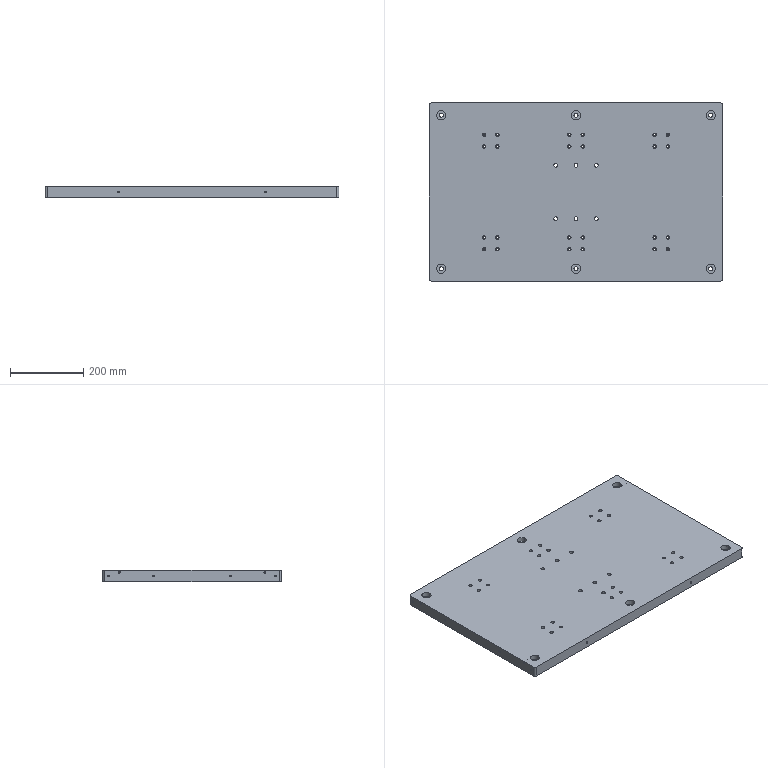NC program | Mastercam | posted with a generic post | part box 800 x 485 x 30 mm
Lines 1 to 630 of 13355:
%
O0000()
(MATERIAL - ALUMINUM MM - 2024)
( T9 | 10 FEM | H9 | XY STOCK TO LEAVE - .2 | Z STOCK TO LEAVE - .05 )
( T10 | 10 FEM | H10 | XY STOCK TO LEAVE - 0. | Z STOCK TO LEAVE - .05 )
( T7 | 6 CHM | H7 )
( T20 | 20 FEM | H20 | XY STOCK TO LEAVE - .15 | Z STOCK TO LEAVE - .1 )
( T1 | 6.8 DR | H1 )
( T18 | 8 DR | H18 )
( T24 | 100 FEM | H24 | XY STOCK TO LEAVE - -1. | Z STOCK TO LEAVE - 0. )
N100 G21
N110 G0 G17 G40 G49 G80 G90
( LRRE )
N120 T9 M6
N130 G0 G90 G54 X-410. Y180.2 A0. S7000 M3
N140 G43 H9 Z50. M8
N150 Z1.
N160 G1 Z-.998 F600.
N170 X-390. F3000.
N180 X-5.
N190 X390.
N200 X410.
N210 Z-1.995 F600.
N220 X390. F3000.
N230 X-5.
N240 X-390.
N250 X-410.
N260 Z-2.993 F600.
N270 X-390. F3000.
N280 X-5.
N290 X390.
N300 X410.
N310 Z-3.99 F600.
N320 X390. F3000.
N330 X-5.
N340 X-390.
N350 X-410.
N360 Z-4.987 F600.
N370 X-390. F3000.
N380 X-5.
N390 X390.
N400 X410.
N410 Z-5.985 F600.
N420 X390. F3000.
N430 X-5.
N440 X-390.
N450 X-410.
N460 Z-6.982 F600.
N470 X-390. F3000.
N480 X-5.
N490 X390.
N500 X410.
N510 Z-7.98 F600.
N520 X390. F3000.
N530 X-5.
N540 X-390.
N550 X-410.
N560 Z-8.977 F600.
N570 X-390. F3000.
N580 X-5.
N590 X390.
N600 X410.
N610 Z-9.975 F600.
N620 X390. F3000.
N630 X-5.
N640 X-390.
N650 X-410.
N660 Z-10.973 F600.
N670 X-390. F3000.
N680 X-5.
N690 X390.
N700 X410.
N710 Z-11.97 F600.
N720 X390. F3000.
N730 X-5.
N740 X-390.
N750 X-410.
N760 Z-12.967 F600.
N770 X-390. F3000.
N780 X-5.
N790 X390.
N800 X410.
N810 Z-13.965 F600.
N820 X390. F3000.
N830 X-5.
N840 X-390.
N850 X-410.
N860 Z-14.963 F600.
N870 X-390. F3000.
N880 X-5.
N890 X390.
N900 X410.
N910 Z-15.96 F600.
N920 X390. F3000.
N930 X-5.
N940 X-390.
N950 X-410.
N960 Z-16.957 F600.
N970 X-390. F3000.
N980 X-5.
N990 X390.
N1000 X410.
N1010 Z-17.955 F600.
N1020 X390. F3000.
N1030 X-5.
N1040 X-390.
N1050 X-410.
N1060 Z-18.953 F600.
N1070 X-390. F3000.
N1080 X-5.
N1090 X390.
N1100 X410.
N1110 Z-19.95 F600.
N1120 X390. F3000.
N1130 X-5.
N1140 X-390.
N1150 X-410.
N1160 G0 Z50.
N1170 X410. Y-180.2
N1180 Z1.
N1190 G1 Z-.998 F600.
N1200 X390. F3000.
N1210 X-5.
N1220 X-390.
N1230 X-410.
N1240 Z-1.995 F600.
N1250 X-390. F3000.
N1260 X-5.
N1270 X390.
N1280 X410.
N1290 Z-2.993 F600.
N1300 X390. F3000.
N1310 X-5.
N1320 X-390.
N1330 X-410.
N1340 Z-3.99 F600.
N1350 X-390. F3000.
N1360 X-5.
N1370 X390.
N1380 X410.
N1390 Z-4.987 F600.
N1400 X390. F3000.
N1410 X-5.
N1420 X-390.
N1430 X-410.
N1440 Z-5.985 F600.
N1450 X-390. F3000.
N1460 X-5.
N1470 X390.
N1480 X410.
N1490 Z-6.982 F600.
N1500 X390. F3000.
N1510 X-5.
N1520 X-390.
N1530 X-410.
N1540 Z-7.98 F600.
N1550 X-390. F3000.
N1560 X-5.
N1570 X390.
N1580 X410.
N1590 Z-8.977 F600.
N1600 X390. F3000.
N1610 X-5.
N1620 X-390.
N1630 X-410.
N1640 Z-9.975 F600.
N1650 X-390. F3000.
N1660 X-5.
N1670 X390.
N1680 X410.
N1690 Z-10.973 F600.
N1700 X390. F3000.
N1710 X-5.
N1720 X-390.
N1730 X-410.
N1740 Z-11.97 F600.
N1750 X-390. F3000.
N1760 X-5.
N1770 X390.
N1780 X410.
N1790 Z-12.967 F600.
N1800 X390. F3000.
N1810 X-5.
N1820 X-390.
N1830 X-410.
N1840 Z-13.965 F600.
N1850 X-390. F3000.
N1860 X-5.
N1870 X390.
N1880 X410.
N1890 Z-14.963 F600.
N1900 X390. F3000.
N1910 X-5.
N1920 X-390.
N1930 X-410.
N1940 Z-15.96 F600.
N1950 X-390. F3000.
N1960 X-5.
N1970 X390.
N1980 X410.
N1990 Z-16.957 F600.
N2000 X390. F3000.
N2010 X-5.
N2020 X-390.
N2030 X-410.
N2040 Z-17.955 F600.
N2050 X-390. F3000.
N2060 X-5.
N2070 X390.
N2080 X410.
N2090 Z-18.953 F600.
N2100 X390. F3000.
N2110 X-5.
N2120 X-390.
N2130 X-410.
N2140 Z-19.95 F600.
N2150 X-390. F3000.
N2160 X-5.
N2170 X390.
N2180 X410.
N2190 G0 Z50.
N2200 M5
N2210 G91 G28 Z0. M9
N2220 A0.
N2230 M01
N2240 T10 M6
N2250 G0 G90 G17 G54 X-410. Y180. A0. S7000 M3
N2260 G43 H10 Z50. M8
N2270 Z1.
N2280 G1 Z-19.95 F600.
N2290 X-390. F1000.
N2300 X-5.
N2310 X390.
N2320 X410.
N2330 G0 Z50.
N2340 Y-180.
N2350 Z1.
N2360 G1 Z-19.95 F600.
N2370 X390. F1000.
N2380 X-5.
N2390 X-390.
N2400 X-410.
N2410 G0 Z50.
N2420 M5
N2430 G91 G28 Z0. M9
N2440 A0.
N2450 M01
N2460 T7 M6
N2470 G0 G90 G17 G54 X-410. Y175.65 A0. S7000 M3
N2480 G43 H7 Z50. M8
N2490 Z1.
N2500 G1 Z-.8 F600.
N2510 X-390. F1000.
N2520 X-5.
N2530 X390.
N2540 X410.
N2550 G0 Z50.
N2560 Y-175.65
N2570 Z1.
N2580 G1 Z-.8 F600.
N2590 X390. F1000.
N2600 X-5.
N2610 X-390.
N2620 X-410.
N2630 G0 Z50.
N2640 M5
N2650 G91 G28 Z0. M9
N2660 A0.
N2670 M01
( LRRECFRBL )
N2680 T9 M6
N2690 G0 G90 G17 G54 X-388. Y-184.2 A0. S7000 M3
N2700 G43 H9 Z50. M8
N2710 Z1.
N2720 G1 Z-.998 F600.
N2730 Y-182.2 F3000.
N2740 G3 X-390. Y-180.2 I-2. J0.
N2750 G2 X-400.2 Y-170. I0. J10.2
N2760 G1 Y170.
N2770 G2 X-390. Y180.2 I10.2 J0.
N2780 G3 X-388. Y182.2 I0. J2.
N2790 G1 Y184.2
N2800 Z-1.995 F600.
N2810 Y182.2 F3000.
N2820 G2 X-390. Y180.2 I-2. J0.
N2830 G3 X-400.2 Y170. I0. J-10.2
N2840 G1 Y-170.
N2850 G3 X-390. Y-180.2 I10.2 J0.
N2860 G2 X-388. Y-182.2 I0. J-2.
N2870 G1 Y-184.2
N2880 Z-2.993 F600.
N2890 Y-182.2 F3000.
N2900 G3 X-390. Y-180.2 I-2. J0.
N2910 G2 X-400.2 Y-170. I0. J10.2
N2920 G1 Y170.
N2930 G2 X-390. Y180.2 I10.2 J0.
N2940 G3 X-388. Y182.2 I0. J2.
N2950 G1 Y184.2
N2960 Z-3.99 F600.
N2970 Y182.2 F3000.
N2980 G2 X-390. Y180.2 I-2. J0.
N2990 G3 X-400.2 Y170. I0. J-10.2
N3000 G1 Y-170.
N3010 G3 X-390. Y-180.2 I10.2 J0.
N3020 G2 X-388. Y-182.2 I0. J-2.
N3030 G1 Y-184.2
N3040 Z-4.987 F600.
N3050 Y-182.2 F3000.
N3060 G3 X-390. Y-180.2 I-2. J0.
N3070 G2 X-400.2 Y-170. I0. J10.2
N3080 G1 Y170.
N3090 G2 X-390. Y180.2 I10.2 J0.
N3100 G3 X-388. Y182.2 I0. J2.
N3110 G1 Y184.2
N3120 Z-5.985 F600.
N3130 Y182.2 F3000.
N3140 G2 X-390. Y180.2 I-2. J0.
N3150 G3 X-400.2 Y170. I0. J-10.2
N3160 G1 Y-170.
N3170 G3 X-390. Y-180.2 I10.2 J0.
N3180 G2 X-388. Y-182.2 I0. J-2.
N3190 G1 Y-184.2
N3200 Z-6.982 F600.
N3210 Y-182.2 F3000.
N3220 G3 X-390. Y-180.2 I-2. J0.
N3230 G2 X-400.2 Y-170. I0. J10.2
N3240 G1 Y170.
N3250 G2 X-390. Y180.2 I10.2 J0.
N3260 G3 X-388. Y182.2 I0. J2.
N3270 G1 Y184.2
N3280 Z-7.98 F600.
N3290 Y182.2 F3000.
N3300 G2 X-390. Y180.2 I-2. J0.
N3310 G3 X-400.2 Y170. I0. J-10.2
N3320 G1 Y-170.
N3330 G3 X-390. Y-180.2 I10.2 J0.
N3340 G2 X-388. Y-182.2 I0. J-2.
N3350 G1 Y-184.2
N3360 Z-8.977 F600.
N3370 Y-182.2 F3000.
N3380 G3 X-390. Y-180.2 I-2. J0.
N3390 G2 X-400.2 Y-170. I0. J10.2
N3400 G1 Y170.
N3410 G2 X-390. Y180.2 I10.2 J0.
N3420 G3 X-388. Y182.2 I0. J2.
N3430 G1 Y184.2
N3440 Z-9.975 F600.
N3450 Y182.2 F3000.
N3460 G2 X-390. Y180.2 I-2. J0.
N3470 G3 X-400.2 Y170. I0. J-10.2
N3480 G1 Y-170.
N3490 G3 X-390. Y-180.2 I10.2 J0.
N3500 G2 X-388. Y-182.2 I0. J-2.
N3510 G1 Y-184.2
N3520 Z-10.973 F600.
N3530 Y-182.2 F3000.
N3540 G3 X-390. Y-180.2 I-2. J0.
N3550 G2 X-400.2 Y-170. I0. J10.2
N3560 G1 Y170.
N3570 G2 X-390. Y180.2 I10.2 J0.
N3580 G3 X-388. Y182.2 I0. J2.
N3590 G1 Y184.2
N3600 Z-11.97 F600.
N3610 Y182.2 F3000.
N3620 G2 X-390. Y180.2 I-2. J0.
N3630 G3 X-400.2 Y170. I0. J-10.2
N3640 G1 Y-170.
N3650 G3 X-390. Y-180.2 I10.2 J0.
N3660 G2 X-388. Y-182.2 I0. J-2.
N3670 G1 Y-184.2
N3680 Z-12.967 F600.
N3690 Y-182.2 F3000.
N3700 G3 X-390. Y-180.2 I-2. J0.
N3710 G2 X-400.2 Y-170. I0. J10.2
N3720 G1 Y170.
N3730 G2 X-390. Y180.2 I10.2 J0.
N3740 G3 X-388. Y182.2 I0. J2.
N3750 G1 Y184.2
N3760 Z-13.965 F600.
N3770 Y182.2 F3000.
N3780 G2 X-390. Y180.2 I-2. J0.
N3790 G3 X-400.2 Y170. I0. J-10.2
N3800 G1 Y-170.
N3810 G3 X-390. Y-180.2 I10.2 J0.
N3820 G2 X-388. Y-182.2 I0. J-2.
N3830 G1 Y-184.2
N3840 Z-14.963 F600.
N3850 Y-182.2 F3000.
N3860 G3 X-390. Y-180.2 I-2. J0.
N3870 G2 X-400.2 Y-170. I0. J10.2
N3880 G1 Y170.
N3890 G2 X-390. Y180.2 I10.2 J0.
N3900 G3 X-388. Y182.2 I0. J2.
N3910 G1 Y184.2
N3920 Z-15.96 F600.
N3930 Y182.2 F3000.
N3940 G2 X-390. Y180.2 I-2. J0.
N3950 G3 X-400.2 Y170. I0. J-10.2
N3960 G1 Y-170.
N3970 G3 X-390. Y-180.2 I10.2 J0.
N3980 G2 X-388. Y-182.2 I0. J-2.
N3990 G1 Y-184.2
N4000 Z-16.957 F600.
N4010 Y-182.2 F3000.
N4020 G3 X-390. Y-180.2 I-2. J0.
N4030 G2 X-400.2 Y-170. I0. J10.2
N4040 G1 Y170.
N4050 G2 X-390. Y180.2 I10.2 J0.
N4060 G3 X-388. Y182.2 I0. J2.
N4070 G1 Y184.2
N4080 Z-17.955 F600.
N4090 Y182.2 F3000.
N4100 G2 X-390. Y180.2 I-2. J0.
N4110 G3 X-400.2 Y170. I0. J-10.2
N4120 G1 Y-170.
N4130 G3 X-390. Y-180.2 I10.2 J0.
N4140 G2 X-388. Y-182.2 I0. J-2.
N4150 G1 Y-184.2
N4160 Z-18.953 F600.
N4170 Y-182.2 F3000.
N4180 G3 X-390. Y-180.2 I-2. J0.
N4190 G2 X-400.2 Y-170. I0. J10.2
N4200 G1 Y170.
N4210 G2 X-390. Y180.2 I10.2 J0.
N4220 G3 X-388. Y182.2 I0. J2.
N4230 G1 Y184.2
N4240 Z-19.95 F600.
N4250 Y182.2 F3000.
N4260 G2 X-390. Y180.2 I-2. J0.
N4270 G3 X-400.2 Y170. I0. J-10.2
N4280 G1 Y-170.
N4290 G3 X-390. Y-180.2 I10.2 J0.
N4300 G2 X-388. Y-182.2 I0. J-2.
N4310 G1 Y-184.2
N4320 G0 Z50.
N4330 X388. Y184.2
N4340 Z1.
N4350 G1 Z-.998 F600.
N4360 Y182.2 F3000.
N4370 G3 X390. Y180.2 I2. J0.
N4380 G2 X400.2 Y170. I0. J-10.2
N4390 G1 Y-170.
N4400 G2 X390. Y-180.2 I-10.2 J0.
N4410 G3 X388. Y-182.2 I0. J-2.
N4420 G1 Y-184.2
N4430 Z-1.995 F600.
N4440 Y-182.2 F3000.
N4450 G2 X390. Y-180.2 I2. J0.
N4460 G3 X400.2 Y-170. I0. J10.2
N4470 G1 Y170.
N4480 G3 X390. Y180.2 I-10.2 J0.
N4490 G2 X388. Y182.2 I0. J2.
N4500 G1 Y184.2
N4510 Z-2.993 F600.
N4520 Y182.2 F3000.
N4530 G3 X390. Y180.2 I2. J0.
N4540 G2 X400.2 Y170. I0. J-10.2
N4550 G1 Y-170.
N4560 G2 X390. Y-180.2 I-10.2 J0.
N4570 G3 X388. Y-182.2 I0. J-2.
N4580 G1 Y-184.2
N4590 Z-3.99 F600.
N4600 Y-182.2 F3000.
N4610 G2 X390. Y-180.2 I2. J0.
N4620 G3 X400.2 Y-170. I0. J10.2
N4630 G1 Y170.
N4640 G3 X390. Y180.2 I-10.2 J0.
N4650 G2 X388. Y182.2 I0. J2.
N4660 G1 Y184.2
N4670 Z-4.987 F600.
N4680 Y182.2 F3000.
N4690 G3 X390. Y180.2 I2. J0.
N4700 G2 X400.2 Y170. I0. J-10.2
N4710 G1 Y-170.
N4720 G2 X390. Y-180.2 I-10.2 J0.
N4730 G3 X388. Y-182.2 I0. J-2.
N4740 G1 Y-184.2
N4750 Z-5.985 F600.
N4760 Y-182.2 F3000.
N4770 G2 X390. Y-180.2 I2. J0.
N4780 G3 X400.2 Y-170. I0. J10.2
N4790 G1 Y170.
N4800 G3 X390. Y180.2 I-10.2 J0.
N4810 G2 X388. Y182.2 I0. J2.
N4820 G1 Y184.2
N4830 Z-6.982 F600.
N4840 Y182.2 F3000.
N4850 G3 X390. Y180.2 I2. J0.
N4860 G2 X400.2 Y170. I0. J-10.2
N4870 G1 Y-170.
N4880 G2 X390. Y-180.2 I-10.2 J0.
N4890 G3 X388. Y-182.2 I0. J-2.
N4900 G1 Y-184.2
N4910 Z-7.98 F600.
N4920 Y-182.2 F3000.
N4930 G2 X390. Y-180.2 I2. J0.
N4940 G3 X400.2 Y-170. I0. J10.2
N4950 G1 Y170.
N4960 G3 X390. Y180.2 I-10.2 J0.
N4970 G2 X388. Y182.2 I0. J2.
N4980 G1 Y184.2
N4990 Z-8.977 F600.
N5000 Y182.2 F3000.
N5010 G3 X390. Y180.2 I2. J0.
N5020 G2 X400.2 Y170. I0. J-10.2
N5030 G1 Y-170.
N5040 G2 X390. Y-180.2 I-10.2 J0.
N5050 G3 X388. Y-182.2 I0. J-2.
N5060 G1 Y-184.2
N5070 Z-9.975 F600.
N5080 Y-182.2 F3000.
N5090 G2 X390. Y-180.2 I2. J0.
N5100 G3 X400.2 Y-170. I0. J10.2
N5110 G1 Y170.
N5120 G3 X390. Y180.2 I-10.2 J0.
N5130 G2 X388. Y182.2 I0. J2.
N5140 G1 Y184.2
N5150 Z-10.973 F600.
N5160 Y182.2 F3000.
N5170 G3 X390. Y180.2 I2. J0.
N5180 G2 X400.2 Y170. I0. J-10.2
N5190 G1 Y-170.
N5200 G2 X390. Y-180.2 I-10.2 J0.
N5210 G3 X388. Y-182.2 I0. J-2.
N5220 G1 Y-184.2
N5230 Z-11.97 F600.
N5240 Y-182.2 F3000.
N5250 G2 X390. Y-180.2 I2. J0.
N5260 G3 X400.2 Y-170. I0. J10.2
N5270 G1 Y170.
N5280 G3 X390. Y180.2 I-10.2 J0.
N5290 G2 X388. Y182.2 I0. J2.
N5300 G1 Y184.2
N5310 Z-12.967 F600.
N5320 Y182.2 F3000.
N5330 G3 X390. Y180.2 I2. J0.
N5340 G2 X400.2 Y170. I0. J-10.2
N5350 G1 Y-170.
N5360 G2 X390. Y-180.2 I-10.2 J0.
N5370 G3 X388. Y-182.2 I0. J-2.
N5380 G1 Y-184.2
N5390 Z-13.965 F600.
N5400 Y-182.2 F3000.
N5410 G2 X390. Y-180.2 I2. J0.
N5420 G3 X400.2 Y-170. I0. J10.2
N5430 G1 Y170.
N5440 G3 X390. Y180.2 I-10.2 J0.
N5450 G2 X388. Y182.2 I0. J2.
N5460 G1 Y184.2
N5470 Z-14.963 F600.
N5480 Y182.2 F3000.
N5490 G3 X390. Y180.2 I2. J0.
N5500 G2 X400.2 Y170. I0. J-10.2
N5510 G1 Y-170.
N5520 G2 X390. Y-180.2 I-10.2 J0.
N5530 G3 X388. Y-182.2 I0. J-2.
N5540 G1 Y-184.2
N5550 Z-15.96 F600.
N5560 Y-182.2 F3000.
N5570 G2 X390. Y-180.2 I2. J0.
N5580 G3 X400.2 Y-170. I0. J10.2
N5590 G1 Y170.
N5600 G3 X390. Y180.2 I-10.2 J0.
N5610 G2 X388. Y182.2 I0. J2.
N5620 G1 Y184.2
N5630 Z-16.957 F600.
N5640 Y182.2 F3000.
N5650 G3 X390. Y180.2 I2. J0.
N5660 G2 X400.2 Y170. I0. J-10.2
N5670 G1 Y-170.
N5680 G2 X390. Y-180.2 I-10.2 J0.
N5690 G3 X388. Y-182.2 I0. J-2.
N5700 G1 Y-184.2
N5710 Z-17.955 F600.
N5720 Y-182.2 F3000.
N5730 G2 X390. Y-180.2 I2. J0.
N5740 G3 X400.2 Y-170. I0. J10.2
N5750 G1 Y170.
N5760 G3 X390. Y180.2 I-10.2 J0.
N5770 G2 X388. Y182.2 I0. J2.
N5780 G1 Y184.2
N5790 Z-18.953 F600.
N5800 Y182.2 F3000.
N5810 G3 X390. Y180.2 I2. J0.
N5820 G2 X400.2 Y170. I0. J-10.2
N5830 G1 Y-170.
N5840 G2 X390. Y-180.2 I-10.2 J0.
N5850 G3 X388. Y-182.2 I0. J-2.
N5860 G1 Y-184.2
N5870 Z-19.95 F600.
N5880 Y-182.2 F3000.
N5890 G2 X390. Y-180.2 I2. J0.
N5900 G3 X400.2 Y-170. I0. J10.2
N5910 G1 Y170.
N5920 G3 X390. Y180.2 I-10.2 J0.
N5930 G2 X388. Y182.2 I0. J2.
N5940 G1 Y184.2
N5950 G0 Z50.
N5960 M5
N5970 G91 G28 Z0. M9
N5980 A0.
N5990 M01
N6000 T10 M6
N6010 G0 G90 G17 G54 X-388. Y-184. A0. S7000 M3
N6020 G43 H10 Z50. M8
N6030 Z1.
N6040 G1 Z-19.95 F600.
N6050 Y-182. F1000.
N6060 G3 X-390. Y-180. I-2. J0.
N6070 G2 X-400. Y-170. I0. J10.
N6080 G1 Y170.
N6090 G2 X-390. Y180. I10. J0.
N6100 G3 X-388. Y182. I0. J2.
N6110 G1 Y184.
N6120 G0 Z50.
N6130 X388.
N6140 Z1.
N6150 G1 Z-19.95 F600.
N6160 Y182. F1000.
N6170 G3 X390. Y180. I2. J0.
N6180 G2 X400. Y170. I0. J-10.
N6190 G1 Y-170.
N6200 G2 X390. Y-180. I-10. J0.
N6210 G3 X388. Y-182. I0. J-2.
N6220 G1 Y-184.
N6230 G0 Z50.
N6240 M5
N6250 G91 G28 Z0. M9
N6260 A0.
N6270 M01